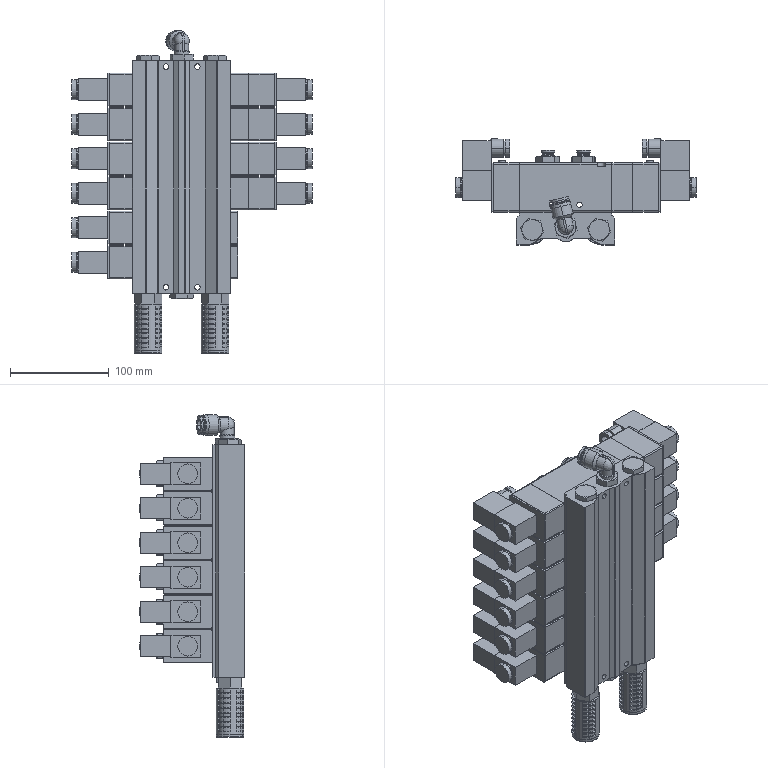Part | SolidWorks | 25 solids | 2631 faces | box 243.8 x 107.3 x 327.5 mm | volume 2539282 mm3 | plane 962 | cylinder 875 | cone 528 | torus 261 | sphere 5 | commonest cylinder face diameters 25 x144 2.4 x140 18.631 x66 11.6 x48 20 x44 15 x40